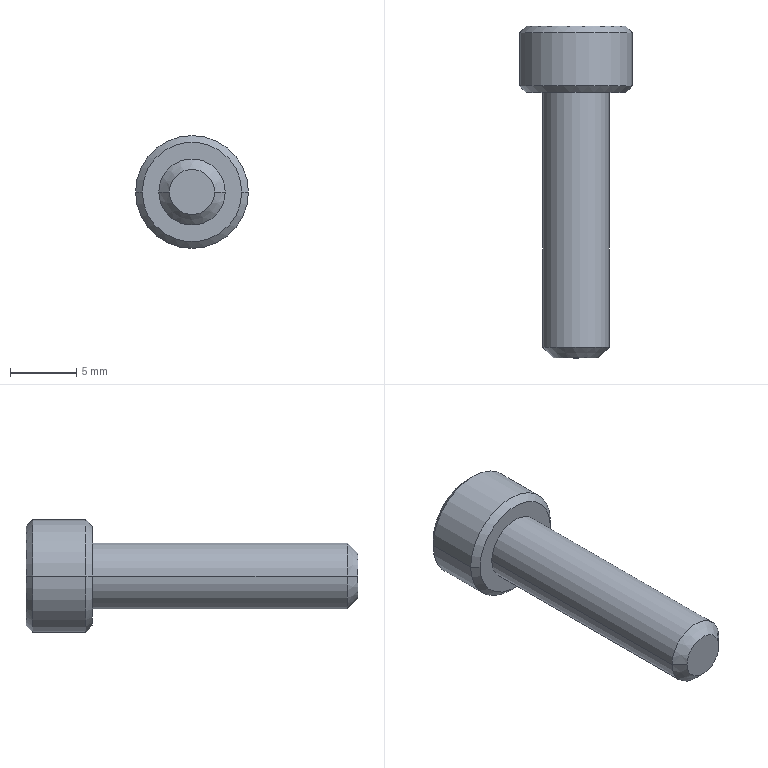Part | STEP file | BB62-M5-20L-1 | 1 solid | 27 faces | box 8.5 x 25 x 8.5 mm | volume 624.198 mm3 | plane 15 | cone 8 | cylinder 4 | commonest cylinder face diameters 5 x2 8.5 x2
STEP:
#1=CARTESIAN_POINT('',(0.,1.178,0.));
#2=VERTEX_POINT('',#1);
#3=CARTESIAN_POINT('',(2.29,2.5,0.));
#4=VERTEX_POINT('',#3);
#5=CARTESIAN_POINT('',(0.,1.178,0.));
#6=DIRECTION('',(0.866,0.5,0.));
#7=VECTOR('',#6,1000.);
#8=LINE('',#5,#7);
#9=EDGE_CURVE('',#2,#4,#8,.T.);
#10=ORIENTED_EDGE('',*,*,#9,.F.);
#11=CARTESIAN_POINT('',(-2.29,2.5,0.));
#12=VERTEX_POINT('',#11);
#13=CARTESIAN_POINT('',(0.,1.178,0.));
#14=DIRECTION('',(-0.866,0.5,0.));
#15=VECTOR('',#14,1000.);
#16=LINE('',#13,#15);
#17=EDGE_CURVE('',#2,#12,#16,.T.);
#18=ORIENTED_EDGE('',*,*,#17,.T.);
#19=CARTESIAN_POINT('',(-1.983,2.5,1.145));
#20=VERTEX_POINT('',#19);
#21=CARTESIAN_POINT('',(0.,2.5,0.));
#22=DIRECTION('',(0.,-1.,0.));
#23=DIRECTION('',(-1.,0.,0.));
#24=AXIS2_PLACEMENT_3D('',#21,#22,#23);
#25=CIRCLE('',#24,2.29);
#26=EDGE_CURVE('',#20,#12,#25,.T.);
#27=ORIENTED_EDGE('',*,*,#26,.F.);
#28=CARTESIAN_POINT('',(0.,2.5,2.29));
#29=VERTEX_POINT('',#28);
#30=CARTESIAN_POINT('',(0.,2.5,0.));
#31=DIRECTION('',(0.,-1.,0.));
#32=DIRECTION('',(-1.,0.,0.));
#33=AXIS2_PLACEMENT_3D('',#30,#31,#32);
#34=CIRCLE('',#33,2.29);
#35=EDGE_CURVE('',#29,#20,#34,.T.);
#36=ORIENTED_EDGE('',*,*,#35,.F.);
#37=CARTESIAN_POINT('',(1.983,2.5,1.145));
#38=VERTEX_POINT('',#37);
#39=CARTESIAN_POINT('',(0.,2.5,0.));
#40=DIRECTION('',(0.,-1.,0.));
#41=DIRECTION('',(-1.,0.,0.));
#42=AXIS2_PLACEMENT_3D('',#39,#40,#41);
#43=CIRCLE('',#42,2.29);
#44=EDGE_CURVE('',#38,#29,#43,.T.);
#45=ORIENTED_EDGE('',*,*,#44,.F.);
#46=CARTESIAN_POINT('',(0.,2.5,0.));
#47=DIRECTION('',(0.,-1.,0.));
#48=DIRECTION('',(-1.,0.,0.));
#49=AXIS2_PLACEMENT_3D('',#46,#47,#48);
#50=CIRCLE('',#49,2.29);
#51=EDGE_CURVE('',#4,#38,#50,.T.);
#52=ORIENTED_EDGE('',*,*,#51,.F.);
#53=EDGE_LOOP('',(#10,#18,#27,#36,#45,#52));
#54=FACE_OUTER_BOUND('',#53,.T.);
#55=CARTESIAN_POINT('',(0.,1001.178,0.));
#56=DIRECTION('',(0.,1.,0.));
#57=DIRECTION('',(1.,0.,0.));
#58=AXIS2_PLACEMENT_3D('',#55,#56,#57);
#59=CONICAL_SURFACE('',#58,1732.051,1.047);
#60=ADVANCED_FACE('',(#54),#59,.F.);
#61=CARTESIAN_POINT('',(1.7,-20.,0.));
#62=VERTEX_POINT('',#61);
#63=CARTESIAN_POINT('',(-1.7,-20.,0.));
#64=VERTEX_POINT('',#63);
#65=CARTESIAN_POINT('',(0.,-20.,0.));
#66=DIRECTION('',(0.,1.,0.));
#67=DIRECTION('',(1.,0.,0.));
#68=AXIS2_PLACEMENT_3D('',#65,#66,#67);
#69=CIRCLE('',#68,1.7);
#70=EDGE_CURVE('',#62,#64,#69,.T.);
#71=ORIENTED_EDGE('',*,*,#70,.T.);
#72=CARTESIAN_POINT('',(-2.5,-19.2,0.));
#73=VERTEX_POINT('',#72);
#74=CARTESIAN_POINT('',(-1.7,-20.,0.));
#75=DIRECTION('',(-0.7071,0.7071,0.));
#76=VECTOR('',#75,1000.);
#77=LINE('',#74,#76);
#78=EDGE_CURVE('',#64,#73,#77,.T.);
#79=ORIENTED_EDGE('',*,*,#78,.T.);
#80=CARTESIAN_POINT('',(2.5,-19.2,0.));
#81=VERTEX_POINT('',#80);
#82=CARTESIAN_POINT('',(0.,-19.2,0.));
#83=DIRECTION('',(0.,-1.,0.));
#84=DIRECTION('',(-1.,0.,0.));
#85=AXIS2_PLACEMENT_3D('',#82,#83,#84);
#86=CIRCLE('',#85,2.5);
#87=EDGE_CURVE('',#73,#81,#86,.T.);
#88=ORIENTED_EDGE('',*,*,#87,.T.);
#89=CARTESIAN_POINT('',(1.7,-20.,0.));
#90=DIRECTION('',(0.7071,0.7071,0.));
#91=VECTOR('',#90,1000.);
#92=LINE('',#89,#91);
#93=EDGE_CURVE('',#62,#81,#92,.T.);
#94=ORIENTED_EDGE('',*,*,#93,.F.);
#95=EDGE_LOOP('',(#71,#79,#88,#94));
#96=FACE_OUTER_BOUND('',#95,.T.);
#97=CARTESIAN_POINT('',(0.,-20.,0.));
#98=DIRECTION('',(0.,1.,0.));
#99=DIRECTION('',(1.,0.,0.));
#100=AXIS2_PLACEMENT_3D('',#97,#98,#99);
#101=CONICAL_SURFACE('',#100,1.7,0.7854);
#102=ADVANCED_FACE('',(#96),#101,.T.);
#103=ORIENTED_EDGE('',*,*,#87,.F.);
#104=CARTESIAN_POINT('',(-2.5,0.,0.));
#105=VERTEX_POINT('',#104);
#106=CARTESIAN_POINT('',(-2.5,-19.2,0.));
#107=DIRECTION('',(0.,1.,0.));
#108=VECTOR('',#107,1000.);
#109=LINE('',#106,#108);
#110=EDGE_CURVE('',#73,#105,#109,.T.);
#111=ORIENTED_EDGE('',*,*,#110,.T.);
#112=CARTESIAN_POINT('',(2.5,0.,0.));
#113=VERTEX_POINT('',#112);
#114=CARTESIAN_POINT('',(0.,0.,0.));
#115=DIRECTION('',(0.,-1.,0.));
#116=DIRECTION('',(-1.,0.,0.));
#117=AXIS2_PLACEMENT_3D('',#114,#115,#116);
#118=CIRCLE('',#117,2.5);
#119=EDGE_CURVE('',#105,#113,#118,.T.);
#120=ORIENTED_EDGE('',*,*,#119,.T.);
#121=CARTESIAN_POINT('',(2.5,-19.2,0.));
#122=DIRECTION('',(0.,1.,0.));
#123=VECTOR('',#122,1000.);
#124=LINE('',#121,#123);
#125=EDGE_CURVE('',#81,#113,#124,.T.);
#126=ORIENTED_EDGE('',*,*,#125,.F.);
#127=EDGE_LOOP('',(#103,#111,#120,#126));
#128=FACE_OUTER_BOUND('',#127,.T.);
#129=CARTESIAN_POINT('',(0.,-19.2,0.));
#130=DIRECTION('',(0.,1.,0.));
#131=DIRECTION('',(1.,0.,0.));
#132=AXIS2_PLACEMENT_3D('',#129,#130,#131);
#133=CYLINDRICAL_SURFACE('',#132,2.5);
#134=ADVANCED_FACE('',(#128),#133,.T.);
#135=CARTESIAN_POINT('',(-3.75,5.,0.));
#136=VERTEX_POINT('',#135);
#137=CARTESIAN_POINT('',(3.75,5.,0.));
#138=VERTEX_POINT('',#137);
#139=CARTESIAN_POINT('',(0.,5.,0.));
#140=DIRECTION('',(0.,-1.,0.));
#141=DIRECTION('',(-1.,0.,0.));
#142=AXIS2_PLACEMENT_3D('',#139,#140,#141);
#143=CIRCLE('',#142,3.75);
#144=EDGE_CURVE('',#136,#138,#143,.T.);
#145=ORIENTED_EDGE('',*,*,#144,.T.);
#146=CARTESIAN_POINT('',(4.25,4.5,0.));
#147=VERTEX_POINT('',#146);
#148=CARTESIAN_POINT('',(4.25,4.5,0.));
#149=DIRECTION('',(0.7071,-0.7071,0.));
#150=VECTOR('',#149,1000.);
#151=LINE('',#148,#150);
#152=EDGE_CURVE('',#138,#147,#151,.T.);
#153=ORIENTED_EDGE('',*,*,#152,.T.);
#154=CARTESIAN_POINT('',(-4.25,4.5,0.));
#155=VERTEX_POINT('',#154);
#156=CARTESIAN_POINT('',(0.,4.5,0.));
#157=DIRECTION('',(0.,-1.,0.));
#158=DIRECTION('',(-1.,0.,0.));
#159=AXIS2_PLACEMENT_3D('',#156,#157,#158);
#160=CIRCLE('',#159,4.25);
#161=EDGE_CURVE('',#155,#147,#160,.T.);
#162=ORIENTED_EDGE('',*,*,#161,.F.);
#163=CARTESIAN_POINT('',(-4.25,4.5,0.));
#164=DIRECTION('',(-0.7071,-0.7071,0.));
#165=VECTOR('',#164,1000.);
#166=LINE('',#163,#165);
#167=EDGE_CURVE('',#136,#155,#166,.T.);
#168=ORIENTED_EDGE('',*,*,#167,.F.);
#169=EDGE_LOOP('',(#145,#153,#162,#168));
#170=FACE_OUTER_BOUND('',#169,.T.);
#171=CARTESIAN_POINT('',(0.,4.5,0.));
#172=DIRECTION('',(0.,-1.,0.));
#173=DIRECTION('',(-1.,0.,0.));
#174=AXIS2_PLACEMENT_3D('',#171,#172,#173);
#175=CONICAL_SURFACE('',#174,4.25,0.7854);
#176=ADVANCED_FACE('',(#170),#175,.T.);
#177=ORIENTED_EDGE('',*,*,#161,.T.);
#178=CARTESIAN_POINT('',(4.25,0.5,0.));
#179=VERTEX_POINT('',#178);
#180=CARTESIAN_POINT('',(4.25,1.62,0.));
#181=DIRECTION('',(0.,-1.,0.));
#182=VECTOR('',#181,1000.);
#183=LINE('',#180,#182);
#184=EDGE_CURVE('',#147,#179,#183,.T.);
#185=ORIENTED_EDGE('',*,*,#184,.T.);
#186=CARTESIAN_POINT('',(-4.25,0.5,0.));
#187=VERTEX_POINT('',#186);
#188=CARTESIAN_POINT('',(0.,0.5,0.));
#189=DIRECTION('',(0.,-1.,0.));
#190=DIRECTION('',(-1.,0.,0.));
#191=AXIS2_PLACEMENT_3D('',#188,#189,#190);
#192=CIRCLE('',#191,4.25);
#193=EDGE_CURVE('',#187,#179,#192,.T.);
#194=ORIENTED_EDGE('',*,*,#193,.F.);
#195=CARTESIAN_POINT('',(-4.25,1.62,0.));
#196=DIRECTION('',(0.,-1.,0.));
#197=VECTOR('',#196,1000.);
#198=LINE('',#195,#197);
#199=EDGE_CURVE('',#155,#187,#198,.T.);
#200=ORIENTED_EDGE('',*,*,#199,.F.);
#201=EDGE_LOOP('',(#177,#185,#194,#200));
#202=FACE_OUTER_BOUND('',#201,.T.);
#203=CARTESIAN_POINT('',(0.,1.62,0.));
#204=DIRECTION('',(0.,-1.,0.));
#205=DIRECTION('',(-1.,0.,0.));
#206=AXIS2_PLACEMENT_3D('',#203,#204,#205);
#207=CYLINDRICAL_SURFACE('',#206,4.25);
#208=ADVANCED_FACE('',(#202),#207,.T.);
#209=CARTESIAN_POINT('',(-3.75,0.,0.));
#210=VERTEX_POINT('',#209);
#211=CARTESIAN_POINT('',(3.75,0.,0.));
#212=VERTEX_POINT('',#211);
#213=CARTESIAN_POINT('',(0.,0.,0.));
#214=DIRECTION('',(0.,-1.,0.));
#215=DIRECTION('',(-1.,0.,0.));
#216=AXIS2_PLACEMENT_3D('',#213,#214,#215);
#217=CIRCLE('',#216,3.75);
#218=EDGE_CURVE('',#210,#212,#217,.T.);
#219=ORIENTED_EDGE('',*,*,#218,.F.);
#220=CARTESIAN_POINT('',(-3.75,0.,0.));
#221=DIRECTION('',(-0.7071,0.7071,0.));
#222=VECTOR('',#221,1000.);
#223=LINE('',#220,#222);
#224=EDGE_CURVE('',#210,#187,#223,.T.);
#225=ORIENTED_EDGE('',*,*,#224,.T.);
#226=ORIENTED_EDGE('',*,*,#193,.T.);
#227=CARTESIAN_POINT('',(3.75,0.,0.));
#228=DIRECTION('',(0.7071,0.7071,0.));
#229=VECTOR('',#228,1000.);
#230=LINE('',#227,#229);
#231=EDGE_CURVE('',#212,#179,#230,.T.);
#232=ORIENTED_EDGE('',*,*,#231,.F.);
#233=EDGE_LOOP('',(#219,#225,#226,#232));
#234=FACE_OUTER_BOUND('',#233,.T.);
#235=CARTESIAN_POINT('',(0.,0.,0.));
#236=DIRECTION('',(0.,1.,0.));
#237=DIRECTION('',(1.,0.,0.));
#238=AXIS2_PLACEMENT_3D('',#235,#236,#237);
#239=CONICAL_SURFACE('',#238,3.75,0.7854);
#240=ADVANCED_FACE('',(#234),#239,.T.);
#241=ORIENTED_EDGE('',*,*,#144,.F.);
#242=CARTESIAN_POINT('',(0.,5.,0.));
#243=DIRECTION('',(0.,-1.,0.));
#244=DIRECTION('',(-1.,0.,0.));
#245=AXIS2_PLACEMENT_3D('',#242,#243,#244);
#246=CIRCLE('',#245,3.75);
#247=EDGE_CURVE('',#138,#136,#246,.T.);
#248=ORIENTED_EDGE('',*,*,#247,.F.);
#249=EDGE_LOOP('',(#241,#248));
#250=FACE_OUTER_BOUND('',#249,.T.);
#251=CARTESIAN_POINT('',(0.,5.,-2.29));
#252=VERTEX_POINT('',#251);
#253=CARTESIAN_POINT('',(-1.983,5.,-1.145));
#254=VERTEX_POINT('',#253);
#255=CARTESIAN_POINT('',(0.,5.,-2.29));
#256=DIRECTION('',(-0.866,0.,0.5));
#257=VECTOR('',#256,1000.);
#258=LINE('',#255,#257);
#259=EDGE_CURVE('',#252,#254,#258,.T.);
#260=ORIENTED_EDGE('',*,*,#259,.F.);
#261=CARTESIAN_POINT('',(1.983,5.,-1.145));
#262=VERTEX_POINT('',#261);
#263=CARTESIAN_POINT('',(1.983,5.,-1.145));
#264=DIRECTION('',(-0.866,0.,-0.5));
#265=VECTOR('',#264,1000.);
#266=LINE('',#263,#265);
#267=EDGE_CURVE('',#262,#252,#266,.T.);
#268=ORIENTED_EDGE('',*,*,#267,.F.);
#269=CARTESIAN_POINT('',(1.983,5.,1.145));
#270=VERTEX_POINT('',#269);
#271=CARTESIAN_POINT('',(1.983,5.,1.145));
#272=DIRECTION('',(0.,0.,-1.));
#273=VECTOR('',#272,1000.);
#274=LINE('',#271,#273);
#275=EDGE_CURVE('',#270,#262,#274,.T.);
#276=ORIENTED_EDGE('',*,*,#275,.F.);
#277=CARTESIAN_POINT('',(0.,5.,2.29));
#278=VERTEX_POINT('',#277);
#279=CARTESIAN_POINT('',(0.,5.,2.29));
#280=DIRECTION('',(0.866,0.,-0.5));
#281=VECTOR('',#280,1000.);
#282=LINE('',#279,#281);
#283=EDGE_CURVE('',#278,#270,#282,.T.);
#284=ORIENTED_EDGE('',*,*,#283,.F.);
#285=CARTESIAN_POINT('',(-1.983,5.,1.145));
#286=VERTEX_POINT('',#285);
#287=CARTESIAN_POINT('',(-1.983,5.,1.145));
#288=DIRECTION('',(0.866,0.,0.5));
#289=VECTOR('',#288,1000.);
#290=LINE('',#287,#289);
#291=EDGE_CURVE('',#286,#278,#290,.T.);
#292=ORIENTED_EDGE('',*,*,#291,.F.);
#293=CARTESIAN_POINT('',(-1.983,5.,-1.145));
#294=DIRECTION('',(0.,0.,1.));
#295=VECTOR('',#294,1000.);
#296=LINE('',#293,#295);
#297=EDGE_CURVE('',#254,#286,#296,.T.);
#298=ORIENTED_EDGE('',*,*,#297,.F.);
#299=EDGE_LOOP('',(#260,#268,#276,#284,#292,#298));
#300=FACE_BOUND('',#299,.T.);
#301=CARTESIAN_POINT('',(3.75,5.,0.));
#302=DIRECTION('',(0.,1.,0.));
#303=DIRECTION('',(1.,0.,0.));
#304=AXIS2_PLACEMENT_3D('',#301,#302,#303);
#305=PLANE('',#304);
#306=ADVANCED_FACE('',(#250,#300),#305,.T.);
#307=CARTESIAN_POINT('',(0.,0.,0.));
#308=DIRECTION('',(0.,-1.,0.));
#309=DIRECTION('',(-1.,0.,0.));
#310=AXIS2_PLACEMENT_3D('',#307,#308,#309);
#311=CIRCLE('',#310,2.5);
#312=EDGE_CURVE('',#113,#105,#311,.T.);
#313=ORIENTED_EDGE('',*,*,#312,.F.);
#314=ORIENTED_EDGE('',*,*,#119,.F.);
#315=EDGE_LOOP('',(#313,#314));
#316=FACE_BOUND('',#315,.T.);
#317=CARTESIAN_POINT('',(0.,0.,0.));
#318=DIRECTION('',(0.,-1.,0.));
#319=DIRECTION('',(-1.,0.,0.));
#320=AXIS2_PLACEMENT_3D('',#317,#318,#319);
#321=CIRCLE('',#320,3.75);
#322=EDGE_CURVE('',#212,#210,#321,.T.);
#323=ORIENTED_EDGE('',*,*,#322,.T.);
#324=ORIENTED_EDGE('',*,*,#218,.T.);
#325=EDGE_LOOP('',(#323,#324));
#326=FACE_OUTER_BOUND('',#325,.T.);
#327=CARTESIAN_POINT('',(0.,0.,0.));
#328=DIRECTION('',(0.,-1.,0.));
#329=DIRECTION('',(-1.,0.,0.));
#330=AXIS2_PLACEMENT_3D('',#327,#328,#329);
#331=PLANE('',#330);
#332=ADVANCED_FACE('',(#316,#326),#331,.T.);
#333=ORIENTED_EDGE('',*,*,#224,.F.);
#334=ORIENTED_EDGE('',*,*,#322,.F.);
#335=ORIENTED_EDGE('',*,*,#231,.T.);
#336=CARTESIAN_POINT('',(0.,0.5,0.));
#337=DIRECTION('',(0.,-1.,0.));
#338=DIRECTION('',(-1.,0.,0.));
#339=AXIS2_PLACEMENT_3D('',#336,#337,#338);
#340=CIRCLE('',#339,4.25);
#341=EDGE_CURVE('',#179,#187,#340,.T.);
#342=ORIENTED_EDGE('',*,*,#341,.T.);
#343=EDGE_LOOP('',(#333,#334,#335,#342));
#344=FACE_OUTER_BOUND('',#343,.T.);
#345=CARTESIAN_POINT('',(0.,0.,0.));
#346=DIRECTION('',(0.,1.,0.));
#347=DIRECTION('',(1.,0.,0.));
#348=AXIS2_PLACEMENT_3D('',#345,#346,#347);
#349=CONICAL_SURFACE('',#348,3.75,0.7854);
#350=ADVANCED_FACE('',(#344),#349,.T.);
#351=ORIENTED_EDGE('',*,*,#184,.F.);
#352=CARTESIAN_POINT('',(0.,4.5,0.));
#353=DIRECTION('',(0.,-1.,0.));
#354=DIRECTION('',(-1.,0.,0.));
#355=AXIS2_PLACEMENT_3D('',#352,#353,#354);
#356=CIRCLE('',#355,4.25);
#357=EDGE_CURVE('',#147,#155,#356,.T.);
#358=ORIENTED_EDGE('',*,*,#357,.T.);
#359=ORIENTED_EDGE('',*,*,#199,.T.);
#360=ORIENTED_EDGE('',*,*,#341,.F.);
#361=EDGE_LOOP('',(#351,#358,#359,#360));
#362=FACE_OUTER_BOUND('',#361,.T.);
#363=CARTESIAN_POINT('',(0.,1.62,0.));
#364=DIRECTION('',(0.,-1.,0.));
#365=DIRECTION('',(-1.,0.,0.));
#366=AXIS2_PLACEMENT_3D('',#363,#364,#365);
#367=CYLINDRICAL_SURFACE('',#366,4.25);
#368=ADVANCED_FACE('',(#362),#367,.T.);
#369=ORIENTED_EDGE('',*,*,#152,.F.);
#370=ORIENTED_EDGE('',*,*,#247,.T.);
#371=ORIENTED_EDGE('',*,*,#167,.T.);
#372=ORIENTED_EDGE('',*,*,#357,.F.);
#373=EDGE_LOOP('',(#369,#370,#371,#372));
#374=FACE_OUTER_BOUND('',#373,.T.);
#375=CARTESIAN_POINT('',(0.,4.5,0.));
#376=DIRECTION('',(0.,-1.,0.));
#377=DIRECTION('',(-1.,0.,0.));
#378=AXIS2_PLACEMENT_3D('',#375,#376,#377);
#379=CONICAL_SURFACE('',#378,4.25,0.7854);
#380=ADVANCED_FACE('',(#374),#379,.T.);
#381=ORIENTED_EDGE('',*,*,#110,.F.);
#382=CARTESIAN_POINT('',(0.,-19.2,0.));
#383=DIRECTION('',(0.,-1.,0.));
#384=DIRECTION('',(-1.,0.,0.));
#385=AXIS2_PLACEMENT_3D('',#382,#383,#384);
#386=CIRCLE('',#385,2.5);
#387=EDGE_CURVE('',#81,#73,#386,.T.);
#388=ORIENTED_EDGE('',*,*,#387,.F.);
#389=ORIENTED_EDGE('',*,*,#125,.T.);
#390=ORIENTED_EDGE('',*,*,#312,.T.);
#391=EDGE_LOOP('',(#381,#388,#389,#390));
#392=FACE_OUTER_BOUND('',#391,.T.);
#393=CARTESIAN_POINT('',(0.,-19.2,0.));
#394=DIRECTION('',(0.,1.,0.));
#395=DIRECTION('',(1.,0.,0.));
#396=AXIS2_PLACEMENT_3D('',#393,#394,#395);
#397=CYLINDRICAL_SURFACE('',#396,2.5);
#398=ADVANCED_FACE('',(#392),#397,.T.);
#399=ORIENTED_EDGE('',*,*,#70,.F.);
#400=CARTESIAN_POINT('',(0.,-20.,0.));
#401=DIRECTION('',(0.,1.,0.));
#402=DIRECTION('',(1.,0.,0.));
#403=AXIS2_PLACEMENT_3D('',#400,#401,#402);
#404=CIRCLE('',#403,1.7);
#405=EDGE_CURVE('',#64,#62,#404,.T.);
#406=ORIENTED_EDGE('',*,*,#405,.F.);
#407=EDGE_LOOP('',(#399,#406));
#408=FACE_OUTER_BOUND('',#407,.T.);
#409=CARTESIAN_POINT('',(0.,-20.,0.));
#410=DIRECTION('',(0.,-1.,0.));
#411=DIRECTION('',(-1.,0.,0.));
#412=AXIS2_PLACEMENT_3D('',#409,#410,#411);
#413=PLANE('',#412);
#414=ADVANCED_FACE('',(#408),#413,.T.);
#415=ORIENTED_EDGE('',*,*,#78,.F.);
#416=ORIENTED_EDGE('',*,*,#405,.T.);
#417=ORIENTED_EDGE('',*,*,#93,.T.);
#418=ORIENTED_EDGE('',*,*,#387,.T.);
#419=EDGE_LOOP('',(#415,#416,#417,#418));
#420=FACE_OUTER_BOUND('',#419,.T.);
#421=CARTESIAN_POINT('',(0.,-20.,0.));
#422=DIRECTION('',(0.,1.,0.));
#423=DIRECTION('',(1.,0.,0.));
#424=AXIS2_PLACEMENT_3D('',#421,#422,#423);
#425=CONICAL_SURFACE('',#424,1.7,0.7854);
#426=ADVANCED_FACE('',(#420),#425,.T.);
#427=CARTESIAN_POINT('',(1.983,2.5,-1.145));
#428=VERTEX_POINT('',#427);
#429=CARTESIAN_POINT('',(0.,2.5,-2.29));
#430=VERTEX_POINT('',#429);
#431=CARTESIAN_POINT('',(1.983,2.5,-1.145));
#432=DIRECTION('',(-0.866,0.,-0.5));
#433=VECTOR('',#432,1000.);
#434=LINE('',#431,#433);
#435=EDGE_CURVE('',#428,#430,#434,.T.);
#436=ORIENTED_EDGE('',*,*,#435,.F.);
#437=CARTESIAN_POINT('',(1.983,5.,-1.145));
#438=DIRECTION('',(0.,-1.,0.));
#439=VECTOR('',#438,1000.);
#440=LINE('',#437,#439);
#441=EDGE_CURVE('',#262,#428,#440,.T.);
#442=ORIENTED_EDGE('',*,*,#441,.F.);
#443=ORIENTED_EDGE('',*,*,#267,.T.);
#444=CARTESIAN_POINT('',(0.,5.,-2.29));
#445=DIRECTION('',(0.,-1.,0.));
#446=VECTOR('',#445,1000.);
#447=LINE('',#444,#446);
#448=EDGE_CURVE('',#252,#430,#447,.T.);
#449=ORIENTED_EDGE('',*,*,#448,.T.);
#450=EDGE_LOOP('',(#436,#442,#443,#449));
#451=FACE_OUTER_BOUND('',#450,.T.);
#452=CARTESIAN_POINT('',(1.983,5.,-1.145));
#453=DIRECTION('',(-0.5,0.,0.866));
#454=DIRECTION('',(0.866,0.,0.5));
#455=AXIS2_PLACEMENT_3D('',#452,#453,#454);
#456=PLANE('',#455);
#457=ADVANCED_FACE('',(#451),#456,.T.);
#458=CARTESIAN_POINT('',(-1.983,2.5,-1.145));
#459=VERTEX_POINT('',#458);
#460=CARTESIAN_POINT('',(0.,2.5,-2.29));
#461=DIRECTION('',(-0.866,0.,0.5));
#462=VECTOR('',#461,1000.);
#463=LINE('',#460,#462);
#464=EDGE_CURVE('',#430,#459,#463,.T.);
#465=ORIENTED_EDGE('',*,*,#464,.F.);
#466=ORIENTED_EDGE('',*,*,#448,.F.);
#467=ORIENTED_EDGE('',*,*,#259,.T.);
#468=CARTESIAN_POINT('',(-1.983,5.,-1.145));
#469=DIRECTION('',(0.,-1.,0.));
#470=VECTOR('',#469,1000.);
#471=LINE('',#468,#470);
#472=EDGE_CURVE('',#254,#459,#471,.T.);
#473=ORIENTED_EDGE('',*,*,#472,.T.);
#474=EDGE_LOOP('',(#465,#466,#467,#473));
#475=FACE_OUTER_BOUND('',#474,.T.);
#476=CARTESIAN_POINT('',(0.,5.,-2.29));
#477=DIRECTION('',(0.5,0.,0.866));
#478=DIRECTION('',(0.866,0.,-0.5));
#479=AXIS2_PLACEMENT_3D('',#476,#477,#478);
#480=PLANE('',#479);
#481=ADVANCED_FACE('',(#475),#480,.T.);
#482=CARTESIAN_POINT('',(-1.983,2.5,-1.145));
#483=DIRECTION('',(0.,0.,1.));
#484=VECTOR('',#483,1000.);
#485=LINE('',#482,#484);
#486=EDGE_CURVE('',#459,#20,#485,.T.);
#487=ORIENTED_EDGE('',*,*,#486,.F.);
#488=ORIENTED_EDGE('',*,*,#472,.F.);
#489=ORIENTED_EDGE('',*,*,#297,.T.);
#490=CARTESIAN_POINT('',(-1.983,5.,1.145));
#491=DIRECTION('',(0.,-1.,0.));
#492=VECTOR('',#491,1000.);
#493=LINE('',#490,#492);
#494=EDGE_CURVE('',#286,#20,#493,.T.);
#495=ORIENTED_EDGE('',*,*,#494,.T.);
#496=EDGE_LOOP('',(#487,#488,#489,#495));
#497=FACE_OUTER_BOUND('',#496,.T.);
#498=CARTESIAN_POINT('',(-1.983,5.,-1.145));
#499=DIRECTION('',(1.,0.,0.));
#500=DIRECTION('',(0.,0.,-1.));
#501=AXIS2_PLACEMENT_3D('',#498,#499,#500);
#502=PLANE('',#501);
#503=ADVANCED_FACE('',(#497),#502,.T.);
#504=CARTESIAN_POINT('',(-1.983,2.5,1.145));
#505=DIRECTION('',(0.866,0.,0.5));
#506=VECTOR('',#505,1000.);
#507=LINE('',#504,#506);
#508=EDGE_CURVE('',#20,#29,#507,.T.);
#509=ORIENTED_EDGE('',*,*,#508,.F.);
#510=ORIENTED_EDGE('',*,*,#494,.F.);
#511=ORIENTED_EDGE('',*,*,#291,.T.);
#512=CARTESIAN_POINT('',(0.,5.,2.29));
#513=DIRECTION('',(0.,-1.,0.));
#514=VECTOR('',#513,1000.);
#515=LINE('',#512,#514);
#516=EDGE_CURVE('',#278,#29,#515,.T.);
#517=ORIENTED_EDGE('',*,*,#516,.T.);
#518=EDGE_LOOP('',(#509,#510,#511,#517));
#519=FACE_OUTER_BOUND('',#518,.T.);
#520=CARTESIAN_POINT('',(-1.983,5.,1.145));
#521=DIRECTION('',(0.5,0.,-0.866));
#522=DIRECTION('',(-0.866,0.,-0.5));
#523=AXIS2_PLACEMENT_3D('',#520,#521,#522);
#524=PLANE('',#523);
#525=ADVANCED_FACE('',(#519),#524,.T.);
#526=CARTESIAN_POINT('',(0.,2.5,2.29));
#527=DIRECTION('',(0.866,0.,-0.5));
#528=VECTOR('',#527,1000.);
#529=LINE('',#526,#528);
#530=EDGE_CURVE('',#29,#38,#529,.T.);
#531=ORIENTED_EDGE('',*,*,#530,.F.);
#532=ORIENTED_EDGE('',*,*,#516,.F.);
#533=ORIENTED_EDGE('',*,*,#283,.T.);
#534=CARTESIAN_POINT('',(1.983,5.,1.145));
#535=DIRECTION('',(0.,-1.,0.));
#536=VECTOR('',#535,1000.);
#537=LINE('',#534,#536);
#538=EDGE_CURVE('',#270,#38,#537,.T.);
#539=ORIENTED_EDGE('',*,*,#538,.T.);
#540=EDGE_LOOP('',(#531,#532,#533,#539));
#541=FACE_OUTER_BOUND('',#540,.T.);
#542=CARTESIAN_POINT('',(0.,5.,2.29));
#543=DIRECTION('',(-0.5,0.,-0.866));
#544=DIRECTION('',(-0.866,0.,0.5));
#545=AXIS2_PLACEMENT_3D('',#542,#543,#544);
#546=PLANE('',#545);
#547=ADVANCED_FACE('',(#541),#546,.T.);
#548=CARTESIAN_POINT('',(1.983,2.5,1.145));
#549=DIRECTION('',(0.,0.,-1.));
#550=VECTOR('',#549,1000.);
#551=LINE('',#548,#550);
#552=EDGE_CURVE('',#38,#428,#551,.T.);
#553=ORIENTED_EDGE('',*,*,#552,.F.);
#554=ORIENTED_EDGE('',*,*,#538,.F.);
#555=ORIENTED_EDGE('',*,*,#275,.T.);
#556=ORIENTED_EDGE('',*,*,#441,.T.);
#557=EDGE_LOOP('',(#553,#554,#555,#556));
#558=FACE_OUTER_BOUND('',#557,.T.);
#559=CARTESIAN_POINT('',(1.983,5.,1.145));
#560=DIRECTION('',(-1.,0.,0.));
#561=DIRECTION('',(0.,0.,1.));
#562=AXIS2_PLACEMENT_3D('',#559,#560,#561);
#563=PLANE('',#562);
#564=ADVANCED_FACE('',(#558),#563,.T.);
#565=ORIENTED_EDGE('',*,*,#435,.T.);
#566=CARTESIAN_POINT('',(0.,2.5,0.));
#567=DIRECTION('',(0.,-1.,0.));
#568=DIRECTION('',(-1.,0.,0.));
#569=AXIS2_PLACEMENT_3D('',#566,#567,#568);
#570=CIRCLE('',#569,2.29);
#571=EDGE_CURVE('',#430,#428,#570,.T.);
#572=ORIENTED_EDGE('',*,*,#571,.T.);
#573=EDGE_LOOP('',(#565,#572));
#574=FACE_OUTER_BOUND('',#573,.T.);
#575=CARTESIAN_POINT('',(0.,2.5,0.));
#576=DIRECTION('',(0.,1.,0.));
#577=DIRECTION('',(1.,0.,0.));
#578=AXIS2_PLACEMENT_3D('',#575,#576,#577);
#579=PLANE('',#578);
#580=ADVANCED_FACE('',(#574),#579,.F.);
#581=ORIENTED_EDGE('',*,*,#552,.T.);
#582=CARTESIAN_POINT('',(0.,2.5,0.));
#583=DIRECTION('',(0.,-1.,0.));
#584=DIRECTION('',(-1.,0.,0.));
#585=AXIS2_PLACEMENT_3D('',#582,#583,#584);
#586=CIRCLE('',#585,2.29);
#587=EDGE_CURVE('',#428,#4,#586,.T.);
#588=ORIENTED_EDGE('',*,*,#587,.T.);
#589=ORIENTED_EDGE('',*,*,#51,.T.);
#590=EDGE_LOOP('',(#581,#588,#589));
#591=FACE_OUTER_BOUND('',#590,.T.);
#592=CARTESIAN_POINT('',(0.,2.5,0.));
#593=DIRECTION('',(0.,1.,0.));
#594=DIRECTION('',(1.,0.,0.));
#595=AXIS2_PLACEMENT_3D('',#592,#593,#594);
#596=PLANE('',#595);
#597=ADVANCED_FACE('',(#591),#596,.F.);
#598=ORIENTED_EDGE('',*,*,#530,.T.);
#599=ORIENTED_EDGE('',*,*,#44,.T.);
#600=EDGE_LOOP('',(#598,#599));
#601=FACE_OUTER_BOUND('',#600,.T.);
#602=CARTESIAN_POINT('',(0.,2.5,0.));
#603=DIRECTION('',(0.,1.,0.));
#604=DIRECTION('',(1.,0.,0.));
#605=AXIS2_PLACEMENT_3D('',#602,#603,#604);
#606=PLANE('',#605);
#607=ADVANCED_FACE('',(#601),#606,.F.);
#608=ORIENTED_EDGE('',*,*,#508,.T.);
#609=ORIENTED_EDGE('',*,*,#35,.T.);
#610=EDGE_LOOP('',(#608,#609));
#611=FACE_OUTER_BOUND('',#610,.T.);
#612=CARTESIAN_POINT('',(0.,2.5,0.));
#613=DIRECTION('',(0.,1.,0.));
#614=DIRECTION('',(1.,0.,0.));
#615=AXIS2_PLACEMENT_3D('',#612,#613,#614);
#616=PLANE('',#615);
#617=ADVANCED_FACE('',(#611),#616,.F.);
#618=ORIENTED_EDGE('',*,*,#486,.T.);
#619=ORIENTED_EDGE('',*,*,#26,.T.);
#620=CARTESIAN_POINT('',(0.,2.5,0.));
#621=DIRECTION('',(0.,-1.,0.));
#622=DIRECTION('',(-1.,0.,0.));
#623=AXIS2_PLACEMENT_3D('',#620,#621,#622);
#624=CIRCLE('',#623,2.29);
#625=EDGE_CURVE('',#12,#459,#624,.T.);
#626=ORIENTED_EDGE('',*,*,#625,.T.);
#627=EDGE_LOOP('',(#618,#619,#626));
#628=FACE_OUTER_BOUND('',#627,.T.);
#629=CARTESIAN_POINT('',(0.,2.5,0.));
#630=DIRECTION('',(0.,1.,0.));
#631=DIRECTION('',(1.,0.,0.));
#632=AXIS2_PLACEMENT_3D('',#629,#630,#631);
#633=PLANE('',#632);
#634=ADVANCED_FACE('',(#628),#633,.F.);
#635=ORIENTED_EDGE('',*,*,#464,.T.);
#636=CARTESIAN_POINT('',(0.,2.5,0.));
#637=DIRECTION('',(0.,-1.,0.));
#638=DIRECTION('',(-1.,0.,0.));
#639=AXIS2_PLACEMENT_3D('',#636,#637,#638);
#640=CIRCLE('',#639,2.29);
#641=EDGE_CURVE('',#459,#430,#640,.T.);
#642=ORIENTED_EDGE('',*,*,#641,.T.);
#643=EDGE_LOOP('',(#635,#642));
#644=FACE_OUTER_BOUND('',#643,.T.);
#645=CARTESIAN_POINT('',(0.,2.5,0.));
#646=DIRECTION('',(0.,1.,0.));
#647=DIRECTION('',(1.,0.,0.));
#648=AXIS2_PLACEMENT_3D('',#645,#646,#647);
#649=PLANE('',#648);
#650=ADVANCED_FACE('',(#644),#649,.F.);
#651=ORIENTED_EDGE('',*,*,#17,.F.);
#652=ORIENTED_EDGE('',*,*,#9,.T.);
#653=ORIENTED_EDGE('',*,*,#587,.F.);
#654=ORIENTED_EDGE('',*,*,#571,.F.);
#655=ORIENTED_EDGE('',*,*,#641,.F.);
#656=ORIENTED_EDGE('',*,*,#625,.F.);
#657=EDGE_LOOP('',(#651,#652,#653,#654,#655,#656));
#658=FACE_OUTER_BOUND('',#657,.T.);
#659=CARTESIAN_POINT('',(0.,1001.178,0.));
#660=DIRECTION('',(0.,1.,0.));
#661=DIRECTION('',(1.,0.,0.));
#662=AXIS2_PLACEMENT_3D('',#659,#660,#661);
#663=CONICAL_SURFACE('',#662,1732.051,1.047);
#664=ADVANCED_FACE('',(#658),#663,.F.);
#665=CLOSED_SHELL('',(#60,#102,#134,#176,#208,#240,#306,#332,#350,#368,#380,#398,#414,#426,#457,#481,#503,#525,#547,#564,#580,#597,#607,#617,#634,#650,#664));
#666=MANIFOLD_SOLID_BREP('',#665);
#667=CARTESIAN_POINT('',(0.,0.,0.));
#668=DIRECTION('',(0.,0.,1.));
#669=DIRECTION('',(1.,0.,0.));
#670=AXIS2_PLACEMENT_3D('',#667,#668,#669);
#671=(LENGTH_UNIT()NAMED_UNIT(*)SI_UNIT(.MILLI.,.METRE.));
#672=UNCERTAINTY_MEASURE_WITH_UNIT(LENGTH_MEASURE(0.00001),#671,'','');
#673=(NAMED_UNIT(*)PLANE_ANGLE_UNIT()SI_UNIT($,.RADIAN.));
#674=(NAMED_UNIT(*)SI_UNIT($,.STERADIAN.)SOLID_ANGLE_UNIT());
#675=(GEOMETRIC_REPRESENTATION_CONTEXT(3)GLOBAL_UNCERTAINTY_ASSIGNED_CONTEXT((#672))GLOBAL_UNIT_ASSIGNED_CONTEXT((#671,#673,#674))REPRESENTATION_CONTEXT('',''));
#676=ADVANCED_BREP_SHAPE_REPRESENTATION('',(#666,#670),#675);